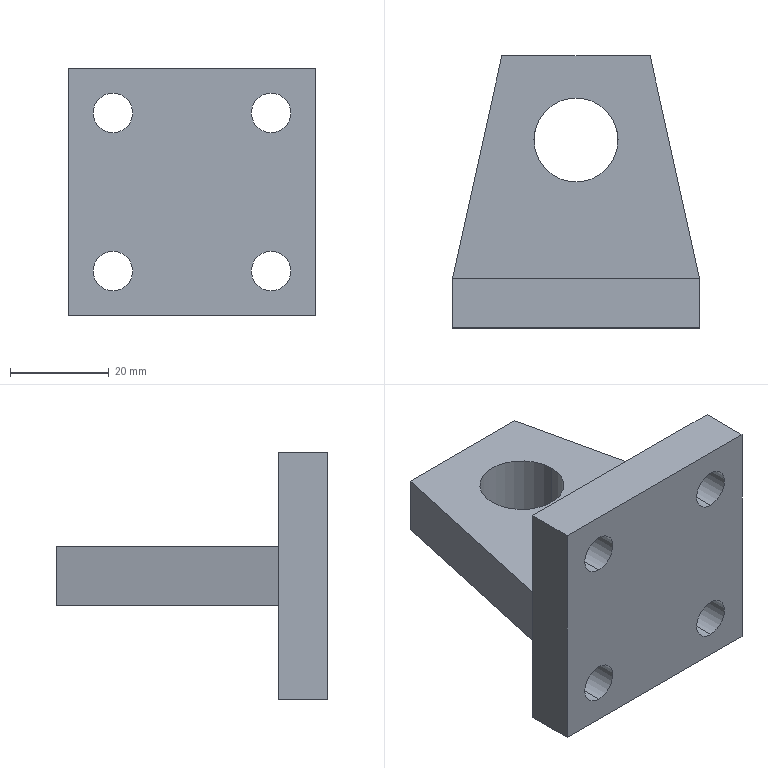Part | STEP file | Do phoi 11 | 2 solids | 22 faces | box 50 x 55 x 50 mm | volume 41866 mm3 | plane 12 | cylinder 10 | commonest cylinder face diameters 8 x8 17 x2